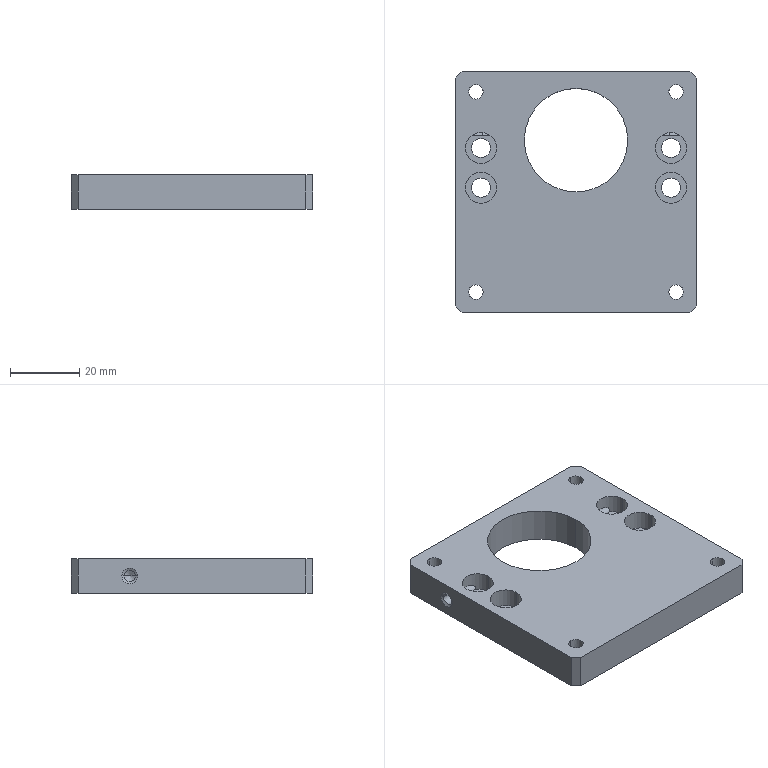Part | NX | 1 solid | 64 faces | box 70 x 70 x 10 mm | volume 39252 mm3 | cylinder 34 | cone 16 | plane 14 | commonest cylinder face diameters 3.3 x8 4.2 x8 5.5 x8 9 x8 30 x2